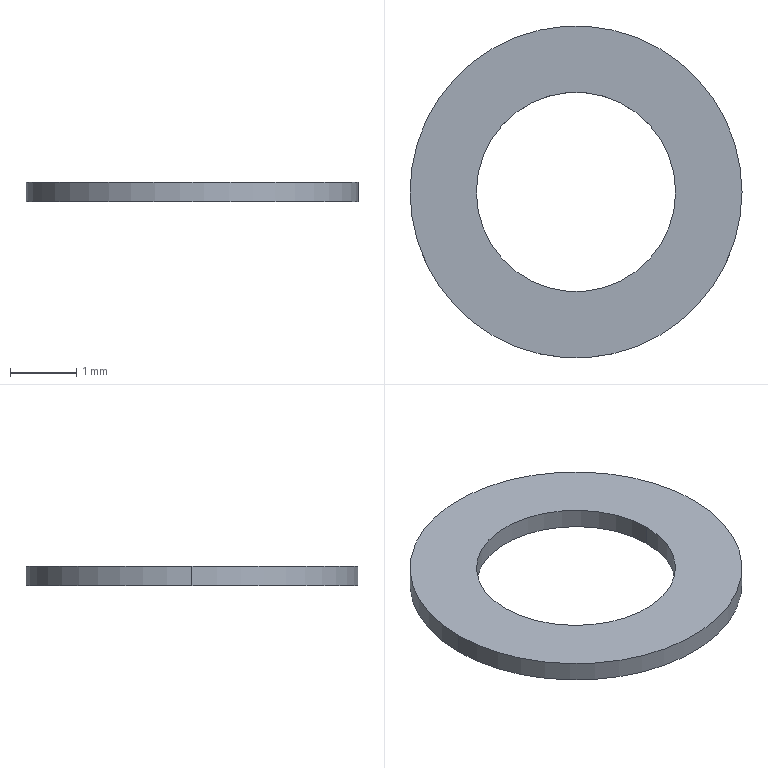Part | SolidWorks | features Extrusion 1, ICE 1 | 1 solid | 6 faces | box 5 x 5 x 0.3 mm | volume 3.77 mm3 | cylinder 4 | plane 2 | commonest cylinder face diameters 3 x2 5 x2
STEP:
#1=CARTESIAN_POINT('',(1.5,0.,0.3));
#2=VERTEX_POINT('',#1);
#3=CARTESIAN_POINT('',(-1.5,0.,0.3));
#4=VERTEX_POINT('',#3);
#5=CARTESIAN_POINT('',(0.,0.,0.3));
#6=DIRECTION('',(0.,0.,-1.));
#7=DIRECTION('',(-1.,0.,0.));
#8=AXIS2_PLACEMENT_3D('',#5,#6,#7);
#9=CIRCLE('',#8,1.5);
#10=EDGE_CURVE('',#2,#4,#9,.T.);
#11=ORIENTED_EDGE('',*,*,#10,.F.);
#12=CARTESIAN_POINT('',(1.5,0.,0.));
#13=VERTEX_POINT('',#12);
#14=CARTESIAN_POINT('',(1.5,0.,0.3));
#15=DIRECTION('',(0.,0.,-1.));
#16=VECTOR('',#15,1000.);
#17=LINE('',#14,#16);
#18=EDGE_CURVE('',#2,#13,#17,.T.);
#19=ORIENTED_EDGE('',*,*,#18,.T.);
#20=CARTESIAN_POINT('',(-1.5,0.,0.));
#21=VERTEX_POINT('',#20);
#22=CARTESIAN_POINT('',(0.,0.,0.));
#23=DIRECTION('',(0.,0.,-1.));
#24=DIRECTION('',(-1.,0.,0.));
#25=AXIS2_PLACEMENT_3D('',#22,#23,#24);
#26=CIRCLE('',#25,1.5);
#27=EDGE_CURVE('',#13,#21,#26,.T.);
#28=ORIENTED_EDGE('',*,*,#27,.T.);
#29=CARTESIAN_POINT('',(-1.5,0.,0.3));
#30=DIRECTION('',(0.,0.,-1.));
#31=VECTOR('',#30,1000.);
#32=LINE('',#29,#31);
#33=EDGE_CURVE('',#4,#21,#32,.T.);
#34=ORIENTED_EDGE('',*,*,#33,.F.);
#35=EDGE_LOOP('',(#11,#19,#28,#34));
#36=FACE_OUTER_BOUND('',#35,.T.);
#37=CARTESIAN_POINT('',(0.,0.,0.3));
#38=DIRECTION('',(0.,0.,-1.));
#39=DIRECTION('',(-1.,0.,0.));
#40=AXIS2_PLACEMENT_3D('',#37,#38,#39);
#41=CYLINDRICAL_SURFACE('',#40,1.5);
#42=ADVANCED_FACE('',(#36),#41,.F.);
#43=CARTESIAN_POINT('',(2.5,0.,0.3));
#44=VERTEX_POINT('',#43);
#45=CARTESIAN_POINT('',(-2.5,0.,0.3));
#46=VERTEX_POINT('',#45);
#47=CARTESIAN_POINT('',(0.,0.,0.3));
#48=DIRECTION('',(0.,0.,1.));
#49=DIRECTION('',(1.,0.,0.));
#50=AXIS2_PLACEMENT_3D('',#47,#48,#49);
#51=CIRCLE('',#50,2.5);
#52=EDGE_CURVE('',#44,#46,#51,.T.);
#53=ORIENTED_EDGE('',*,*,#52,.F.);
#54=CARTESIAN_POINT('',(2.5,0.,0.));
#55=VERTEX_POINT('',#54);
#56=CARTESIAN_POINT('',(2.5,0.,0.3));
#57=DIRECTION('',(0.,0.,-1.));
#58=VECTOR('',#57,1000.);
#59=LINE('',#56,#58);
#60=EDGE_CURVE('',#44,#55,#59,.T.);
#61=ORIENTED_EDGE('',*,*,#60,.T.);
#62=CARTESIAN_POINT('',(-2.5,0.,0.));
#63=VERTEX_POINT('',#62);
#64=CARTESIAN_POINT('',(0.,0.,0.));
#65=DIRECTION('',(0.,0.,1.));
#66=DIRECTION('',(1.,0.,0.));
#67=AXIS2_PLACEMENT_3D('',#64,#65,#66);
#68=CIRCLE('',#67,2.5);
#69=EDGE_CURVE('',#55,#63,#68,.T.);
#70=ORIENTED_EDGE('',*,*,#69,.T.);
#71=CARTESIAN_POINT('',(-2.5,0.,0.3));
#72=DIRECTION('',(0.,0.,-1.));
#73=VECTOR('',#72,1000.);
#74=LINE('',#71,#73);
#75=EDGE_CURVE('',#46,#63,#74,.T.);
#76=ORIENTED_EDGE('',*,*,#75,.F.);
#77=EDGE_LOOP('',(#53,#61,#70,#76));
#78=FACE_OUTER_BOUND('',#77,.T.);
#79=CARTESIAN_POINT('',(0.,0.,0.3));
#80=DIRECTION('',(0.,0.,-1.));
#81=DIRECTION('',(-1.,0.,0.));
#82=AXIS2_PLACEMENT_3D('',#79,#80,#81);
#83=CYLINDRICAL_SURFACE('',#82,2.5);
#84=ADVANCED_FACE('',(#78),#83,.T.);
#85=ORIENTED_EDGE('',*,*,#60,.F.);
#86=CARTESIAN_POINT('',(0.,0.,0.3));
#87=DIRECTION('',(0.,0.,1.));
#88=DIRECTION('',(1.,0.,0.));
#89=AXIS2_PLACEMENT_3D('',#86,#87,#88);
#90=CIRCLE('',#89,2.5);
#91=EDGE_CURVE('',#46,#44,#90,.T.);
#92=ORIENTED_EDGE('',*,*,#91,.F.);
#93=ORIENTED_EDGE('',*,*,#75,.T.);
#94=CARTESIAN_POINT('',(0.,0.,0.));
#95=DIRECTION('',(0.,0.,1.));
#96=DIRECTION('',(1.,0.,0.));
#97=AXIS2_PLACEMENT_3D('',#94,#95,#96);
#98=CIRCLE('',#97,2.5);
#99=EDGE_CURVE('',#63,#55,#98,.T.);
#100=ORIENTED_EDGE('',*,*,#99,.T.);
#101=EDGE_LOOP('',(#85,#92,#93,#100));
#102=FACE_OUTER_BOUND('',#101,.T.);
#103=CARTESIAN_POINT('',(0.,0.,0.3));
#104=DIRECTION('',(0.,0.,-1.));
#105=DIRECTION('',(-1.,0.,0.));
#106=AXIS2_PLACEMENT_3D('',#103,#104,#105);
#107=CYLINDRICAL_SURFACE('',#106,2.5);
#108=ADVANCED_FACE('',(#102),#107,.T.);
#109=CARTESIAN_POINT('',(0.,0.,0.3));
#110=DIRECTION('',(0.,0.,-1.));
#111=DIRECTION('',(-1.,0.,0.));
#112=AXIS2_PLACEMENT_3D('',#109,#110,#111);
#113=CIRCLE('',#112,1.5);
#114=EDGE_CURVE('',#4,#2,#113,.T.);
#115=ORIENTED_EDGE('',*,*,#114,.T.);
#116=ORIENTED_EDGE('',*,*,#10,.T.);
#117=EDGE_LOOP('',(#115,#116));
#118=FACE_BOUND('',#117,.T.);
#119=ORIENTED_EDGE('',*,*,#91,.T.);
#120=ORIENTED_EDGE('',*,*,#52,.T.);
#121=EDGE_LOOP('',(#119,#120));
#122=FACE_OUTER_BOUND('',#121,.T.);
#123=CARTESIAN_POINT('',(0.,0.,0.3));
#124=DIRECTION('',(0.,0.,1.));
#125=DIRECTION('',(1.,0.,0.));
#126=AXIS2_PLACEMENT_3D('',#123,#124,#125);
#127=PLANE('',#126);
#128=ADVANCED_FACE('',(#118,#122),#127,.T.);
#129=CARTESIAN_POINT('',(0.,0.,0.));
#130=DIRECTION('',(0.,0.,-1.));
#131=DIRECTION('',(-1.,0.,0.));
#132=AXIS2_PLACEMENT_3D('',#129,#130,#131);
#133=CIRCLE('',#132,1.5);
#134=EDGE_CURVE('',#21,#13,#133,.T.);
#135=ORIENTED_EDGE('',*,*,#134,.F.);
#136=ORIENTED_EDGE('',*,*,#27,.F.);
#137=EDGE_LOOP('',(#135,#136));
#138=FACE_BOUND('',#137,.T.);
#139=ORIENTED_EDGE('',*,*,#99,.F.);
#140=ORIENTED_EDGE('',*,*,#69,.F.);
#141=EDGE_LOOP('',(#139,#140));
#142=FACE_OUTER_BOUND('',#141,.T.);
#143=CARTESIAN_POINT('',(0.,0.,0.));
#144=DIRECTION('',(0.,0.,1.));
#145=DIRECTION('',(1.,0.,0.));
#146=AXIS2_PLACEMENT_3D('',#143,#144,#145);
#147=PLANE('',#146);
#148=ADVANCED_FACE('',(#138,#142),#147,.F.);
#149=ORIENTED_EDGE('',*,*,#18,.F.);
#150=ORIENTED_EDGE('',*,*,#114,.F.);
#151=ORIENTED_EDGE('',*,*,#33,.T.);
#152=ORIENTED_EDGE('',*,*,#134,.T.);
#153=EDGE_LOOP('',(#149,#150,#151,#152));
#154=FACE_OUTER_BOUND('',#153,.T.);
#155=CARTESIAN_POINT('',(0.,0.,0.3));
#156=DIRECTION('',(0.,0.,-1.));
#157=DIRECTION('',(-1.,0.,0.));
#158=AXIS2_PLACEMENT_3D('',#155,#156,#157);
#159=CYLINDRICAL_SURFACE('',#158,1.5);
#160=ADVANCED_FACE('',(#154),#159,.F.);
#161=CLOSED_SHELL('',(#42,#84,#108,#128,#148,#160));
#162=MANIFOLD_SOLID_BREP('',#161);
#163=CARTESIAN_POINT('',(0.,0.,0.));
#164=DIRECTION('',(0.,0.,1.));
#165=DIRECTION('',(1.,0.,0.));
#166=AXIS2_PLACEMENT_3D('',#163,#164,#165);
#167=(LENGTH_UNIT()NAMED_UNIT(*)SI_UNIT(.MILLI.,.METRE.));
#168=UNCERTAINTY_MEASURE_WITH_UNIT(LENGTH_MEASURE(0.00001),#167,'','');
#169=(NAMED_UNIT(*)PLANE_ANGLE_UNIT()SI_UNIT($,.RADIAN.));
#170=(NAMED_UNIT(*)SI_UNIT($,.STERADIAN.)SOLID_ANGLE_UNIT());
#171=(GEOMETRIC_REPRESENTATION_CONTEXT(3)GLOBAL_UNCERTAINTY_ASSIGNED_CONTEXT((#168))GLOBAL_UNIT_ASSIGNED_CONTEXT((#167,#169,#170))REPRESENTATION_CONTEXT('',''));
#172=ADVANCED_BREP_SHAPE_REPRESENTATION('',(#162,#166),#171);